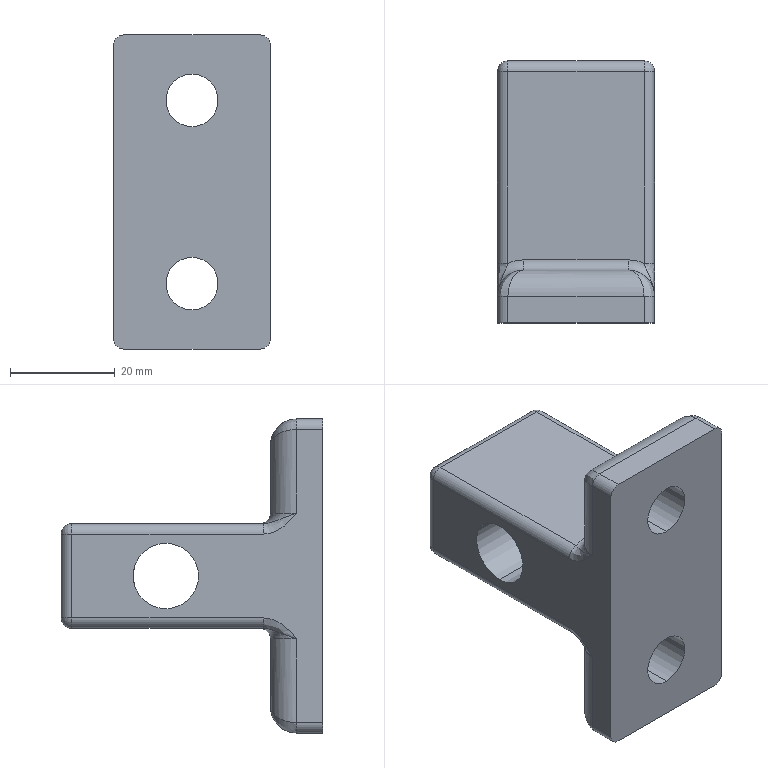Part | SolidWorks | features HoleWzd 3, Fillet 2, ICE 2, Chamfer 1, Extrusion 1 | 1 solid | 56 faces | box 30 x 50 x 60 mm | volume 35816 mm3 | cylinder 28 | plane 10 | spline 8 | torus 4 | sphere 4 | cone 2 | commonest cylinder face diameters 4 x14 10 x10 1.778 x2 12.5 x2